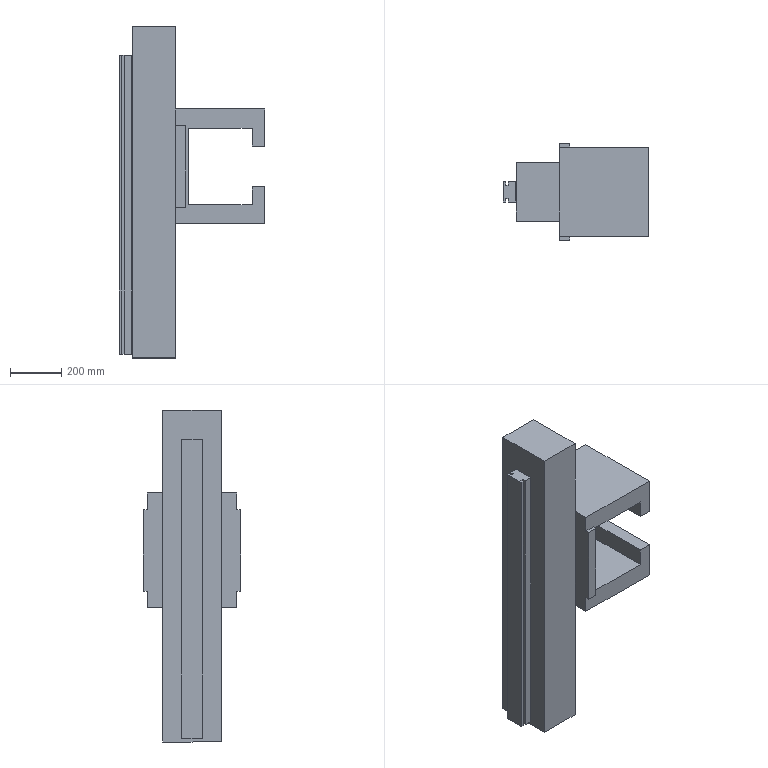Part | SolidWorks | features ICE 4, Extrusion 1 | 2 solids | 44 faces | box 571 x 380 x 1300 mm | volume 81618000 mm3 | plane 44
STEP:
#1=CARTESIAN_POINT('',(-175.,290.,550.));
#2=VERTEX_POINT('',#1);
#3=CARTESIAN_POINT('',(-345.,290.,550.));
#4=VERTEX_POINT('',#3);
#5=CARTESIAN_POINT('',(-345.,290.,550.));
#6=DIRECTION('',(-1.,0.,0.));
#7=VECTOR('',#6,1000.);
#8=LINE('',#5,#7);
#9=EDGE_CURVE('',#2,#4,#8,.T.);
#10=ORIENTED_EDGE('',*,*,#9,.F.);
#11=CARTESIAN_POINT('',(-175.,290.,225.));
#12=VERTEX_POINT('',#11);
#13=CARTESIAN_POINT('',(-175.,290.,-750.));
#14=DIRECTION('',(0.,0.,-1.));
#15=VECTOR('',#14,1000.);
#16=LINE('',#13,#15);
#17=EDGE_CURVE('',#2,#12,#16,.T.);
#18=ORIENTED_EDGE('',*,*,#17,.T.);
#19=CARTESIAN_POINT('',(-175.,290.,-225.));
#20=VERTEX_POINT('',#19);
#21=CARTESIAN_POINT('',(-175.,290.,-750.));
#22=DIRECTION('',(0.,0.,-1.));
#23=VECTOR('',#22,1000.);
#24=LINE('',#21,#23);
#25=EDGE_CURVE('',#12,#20,#24,.T.);
#26=ORIENTED_EDGE('',*,*,#25,.T.);
#27=CARTESIAN_POINT('',(-175.,290.,-750.));
#28=VERTEX_POINT('',#27);
#29=CARTESIAN_POINT('',(-175.,290.,-750.));
#30=DIRECTION('',(0.,0.,-1.));
#31=VECTOR('',#30,1000.);
#32=LINE('',#29,#31);
#33=EDGE_CURVE('',#20,#28,#32,.T.);
#34=ORIENTED_EDGE('',*,*,#33,.T.);
#35=CARTESIAN_POINT('',(-345.,290.,-750.));
#36=VERTEX_POINT('',#35);
#37=CARTESIAN_POINT('',(-345.,290.,-750.));
#38=DIRECTION('',(1.,0.,0.));
#39=VECTOR('',#38,1000.);
#40=LINE('',#37,#39);
#41=EDGE_CURVE('',#36,#28,#40,.T.);
#42=ORIENTED_EDGE('',*,*,#41,.F.);
#43=CARTESIAN_POINT('',(-345.,290.,-750.));
#44=DIRECTION('',(0.,0.,-1.));
#45=VECTOR('',#44,1000.);
#46=LINE('',#43,#45);
#47=EDGE_CURVE('',#4,#36,#46,.T.);
#48=ORIENTED_EDGE('',*,*,#47,.F.);
#49=EDGE_LOOP('',(#10,#18,#26,#34,#42,#48));
#50=FACE_OUTER_BOUND('',#49,.T.);
#51=CARTESIAN_POINT('',(-345.,290.,-750.));
#52=DIRECTION('',(0.,-1.,0.));
#53=DIRECTION('',(0.,0.,-1.));
#54=AXIS2_PLACEMENT_3D('',#51,#52,#53);
#55=PLANE('',#54);
#56=ADVANCED_FACE('',(#50),#55,.F.);
#57=CARTESIAN_POINT('',(-345.,60.,550.));
#58=VERTEX_POINT('',#57);
#59=CARTESIAN_POINT('',(-175.,60.,550.));
#60=VERTEX_POINT('',#59);
#61=CARTESIAN_POINT('',(-345.,60.,550.));
#62=DIRECTION('',(1.,0.,0.));
#63=VECTOR('',#62,1000.);
#64=LINE('',#61,#63);
#65=EDGE_CURVE('',#58,#60,#64,.T.);
#66=ORIENTED_EDGE('',*,*,#65,.F.);
#67=CARTESIAN_POINT('',(-345.,60.,-750.));
#68=VERTEX_POINT('',#67);
#69=CARTESIAN_POINT('',(-345.,60.,-750.));
#70=DIRECTION('',(0.,0.,1.));
#71=VECTOR('',#70,1000.);
#72=LINE('',#69,#71);
#73=EDGE_CURVE('',#68,#58,#72,.T.);
#74=ORIENTED_EDGE('',*,*,#73,.F.);
#75=CARTESIAN_POINT('',(-175.,60.,-750.));
#76=VERTEX_POINT('',#75);
#77=CARTESIAN_POINT('',(-345.,60.,-750.));
#78=DIRECTION('',(1.,0.,0.));
#79=VECTOR('',#78,1000.);
#80=LINE('',#77,#79);
#81=EDGE_CURVE('',#68,#76,#80,.T.);
#82=ORIENTED_EDGE('',*,*,#81,.T.);
#83=CARTESIAN_POINT('',(-175.,60.,-225.));
#84=VERTEX_POINT('',#83);
#85=CARTESIAN_POINT('',(-175.,60.,-750.));
#86=DIRECTION('',(0.,0.,1.));
#87=VECTOR('',#86,1000.);
#88=LINE('',#85,#87);
#89=EDGE_CURVE('',#76,#84,#88,.T.);
#90=ORIENTED_EDGE('',*,*,#89,.T.);
#91=CARTESIAN_POINT('',(-175.,60.,225.));
#92=VERTEX_POINT('',#91);
#93=CARTESIAN_POINT('',(-175.,60.,-750.));
#94=DIRECTION('',(0.,0.,1.));
#95=VECTOR('',#94,1000.);
#96=LINE('',#93,#95);
#97=EDGE_CURVE('',#84,#92,#96,.T.);
#98=ORIENTED_EDGE('',*,*,#97,.T.);
#99=CARTESIAN_POINT('',(-175.,60.,-750.));
#100=DIRECTION('',(0.,0.,1.));
#101=VECTOR('',#100,1000.);
#102=LINE('',#99,#101);
#103=EDGE_CURVE('',#92,#60,#102,.T.);
#104=ORIENTED_EDGE('',*,*,#103,.T.);
#105=EDGE_LOOP('',(#66,#74,#82,#90,#98,#104));
#106=FACE_OUTER_BOUND('',#105,.T.);
#107=CARTESIAN_POINT('',(-345.,60.,-750.));
#108=DIRECTION('',(0.,1.,0.));
#109=DIRECTION('',(0.,0.,1.));
#110=AXIS2_PLACEMENT_3D('',#107,#108,#109);
#111=PLANE('',#110);
#112=ADVANCED_FACE('',(#106),#111,.F.);
#113=ORIENTED_EDGE('',*,*,#73,.T.);
#114=CARTESIAN_POINT('',(-345.,0.,550.));
#115=DIRECTION('',(0.,1.,0.));
#116=VECTOR('',#115,1000.);
#117=LINE('',#114,#116);
#118=EDGE_CURVE('',#58,#4,#117,.T.);
#119=ORIENTED_EDGE('',*,*,#118,.T.);
#120=ORIENTED_EDGE('',*,*,#47,.T.);
#121=CARTESIAN_POINT('',(-345.,290.,-750.));
#122=DIRECTION('',(0.,-1.,0.));
#123=VECTOR('',#122,1000.);
#124=LINE('',#121,#123);
#125=EDGE_CURVE('',#36,#68,#124,.T.);
#126=ORIENTED_EDGE('',*,*,#125,.T.);
#127=EDGE_LOOP('',(#113,#119,#120,#126));
#128=FACE_OUTER_BOUND('',#127,.T.);
#129=CARTESIAN_POINT('',(-345.,0.,0.));
#130=DIRECTION('',(-1.,0.,0.));
#131=DIRECTION('',(0.,0.,1.));
#132=AXIS2_PLACEMENT_3D('',#129,#130,#131);
#133=PLANE('',#132);
#134=ADVANCED_FACE('',(#128),#133,.T.);
#135=CARTESIAN_POINT('',(-175.,0.,550.));
#136=DIRECTION('',(0.,1.,0.));
#137=VECTOR('',#136,1000.);
#138=LINE('',#135,#137);
#139=EDGE_CURVE('',#60,#2,#138,.T.);
#140=ORIENTED_EDGE('',*,*,#139,.F.);
#141=ORIENTED_EDGE('',*,*,#103,.F.);
#142=CARTESIAN_POINT('',(-175.,350.,225.));
#143=DIRECTION('',(0.,-1.,0.));
#144=VECTOR('',#143,1000.);
#145=LINE('',#142,#144);
#146=EDGE_CURVE('',#12,#92,#145,.T.);
#147=ORIENTED_EDGE('',*,*,#146,.F.);
#148=ORIENTED_EDGE('',*,*,#17,.F.);
#149=EDGE_LOOP('',(#140,#141,#147,#148));
#150=FACE_OUTER_BOUND('',#149,.T.);
#151=CARTESIAN_POINT('',(-175.,0.,0.));
#152=DIRECTION('',(-1.,0.,0.));
#153=DIRECTION('',(0.,0.,1.));
#154=AXIS2_PLACEMENT_3D('',#151,#152,#153);
#155=PLANE('',#154);
#156=ADVANCED_FACE('',(#150),#155,.F.);
#157=ORIENTED_EDGE('',*,*,#97,.F.);
#158=CARTESIAN_POINT('',(-175.,0.,-225.));
#159=VERTEX_POINT('',#158);
#160=CARTESIAN_POINT('',(-175.,350.,-225.));
#161=DIRECTION('',(0.,-1.,0.));
#162=VECTOR('',#161,1000.);
#163=LINE('',#160,#162);
#164=EDGE_CURVE('',#84,#159,#163,.T.);
#165=ORIENTED_EDGE('',*,*,#164,.T.);
#166=CARTESIAN_POINT('',(-175.,0.,-160.));
#167=VERTEX_POINT('',#166);
#168=CARTESIAN_POINT('',(-175.,0.,-225.));
#169=DIRECTION('',(0.,0.,1.));
#170=VECTOR('',#169,1000.);
#171=LINE('',#168,#170);
#172=EDGE_CURVE('',#159,#167,#171,.T.);
#173=ORIENTED_EDGE('',*,*,#172,.T.);
#174=CARTESIAN_POINT('',(-175.,-15.,-160.));
#175=VERTEX_POINT('',#174);
#176=CARTESIAN_POINT('',(-175.,365.,-160.));
#177=DIRECTION('',(0.,-1.,0.));
#178=VECTOR('',#177,1000.);
#179=LINE('',#176,#178);
#180=EDGE_CURVE('',#167,#175,#179,.T.);
#181=ORIENTED_EDGE('',*,*,#180,.T.);
#182=CARTESIAN_POINT('',(-175.,-15.,160.));
#183=VERTEX_POINT('',#182);
#184=CARTESIAN_POINT('',(-175.,-15.,-160.));
#185=DIRECTION('',(0.,0.,1.));
#186=VECTOR('',#185,1000.);
#187=LINE('',#184,#186);
#188=EDGE_CURVE('',#175,#183,#187,.T.);
#189=ORIENTED_EDGE('',*,*,#188,.T.);
#190=CARTESIAN_POINT('',(-175.,0.,160.));
#191=VERTEX_POINT('',#190);
#192=CARTESIAN_POINT('',(-175.,365.,160.));
#193=DIRECTION('',(0.,1.,0.));
#194=VECTOR('',#193,1000.);
#195=LINE('',#192,#194);
#196=EDGE_CURVE('',#183,#191,#195,.T.);
#197=ORIENTED_EDGE('',*,*,#196,.T.);
#198=CARTESIAN_POINT('',(-175.,0.,225.));
#199=VERTEX_POINT('',#198);
#200=CARTESIAN_POINT('',(-175.,0.,-225.));
#201=DIRECTION('',(0.,0.,1.));
#202=VECTOR('',#201,1000.);
#203=LINE('',#200,#202);
#204=EDGE_CURVE('',#191,#199,#203,.T.);
#205=ORIENTED_EDGE('',*,*,#204,.T.);
#206=CARTESIAN_POINT('',(-175.,350.,225.));
#207=DIRECTION('',(0.,-1.,0.));
#208=VECTOR('',#207,1000.);
#209=LINE('',#206,#208);
#210=EDGE_CURVE('',#92,#199,#209,.T.);
#211=ORIENTED_EDGE('',*,*,#210,.F.);
#212=EDGE_LOOP('',(#157,#165,#173,#181,#189,#197,#205,#211));
#213=FACE_OUTER_BOUND('',#212,.T.);
#214=CARTESIAN_POINT('',(-175.,350.,-225.));
#215=DIRECTION('',(1.,0.,0.));
#216=DIRECTION('',(0.,0.,-1.));
#217=AXIS2_PLACEMENT_3D('',#214,#215,#216);
#218=PLANE('',#217);
#219=ADVANCED_FACE('',(#213),#218,.F.);
#220=ORIENTED_EDGE('',*,*,#25,.F.);
#221=CARTESIAN_POINT('',(-175.,350.,225.));
#222=VERTEX_POINT('',#221);
#223=CARTESIAN_POINT('',(-175.,350.,225.));
#224=DIRECTION('',(0.,-1.,0.));
#225=VECTOR('',#224,1000.);
#226=LINE('',#223,#225);
#227=EDGE_CURVE('',#222,#12,#226,.T.);
#228=ORIENTED_EDGE('',*,*,#227,.F.);
#229=CARTESIAN_POINT('',(-175.,350.,160.));
#230=VERTEX_POINT('',#229);
#231=CARTESIAN_POINT('',(-175.,350.,-225.));
#232=DIRECTION('',(0.,0.,1.));
#233=VECTOR('',#232,1000.);
#234=LINE('',#231,#233);
#235=EDGE_CURVE('',#230,#222,#234,.T.);
#236=ORIENTED_EDGE('',*,*,#235,.F.);
#237=CARTESIAN_POINT('',(-175.,365.,160.));
#238=VERTEX_POINT('',#237);
#239=CARTESIAN_POINT('',(-175.,365.,160.));
#240=DIRECTION('',(0.,1.,0.));
#241=VECTOR('',#240,1000.);
#242=LINE('',#239,#241);
#243=EDGE_CURVE('',#230,#238,#242,.T.);
#244=ORIENTED_EDGE('',*,*,#243,.T.);
#245=CARTESIAN_POINT('',(-175.,365.,-160.));
#246=VERTEX_POINT('',#245);
#247=CARTESIAN_POINT('',(-175.,365.,-160.));
#248=DIRECTION('',(0.,0.,-1.));
#249=VECTOR('',#248,1000.);
#250=LINE('',#247,#249);
#251=EDGE_CURVE('',#238,#246,#250,.T.);
#252=ORIENTED_EDGE('',*,*,#251,.T.);
#253=CARTESIAN_POINT('',(-175.,350.,-160.));
#254=VERTEX_POINT('',#253);
#255=CARTESIAN_POINT('',(-175.,365.,-160.));
#256=DIRECTION('',(0.,-1.,0.));
#257=VECTOR('',#256,1000.);
#258=LINE('',#255,#257);
#259=EDGE_CURVE('',#246,#254,#258,.T.);
#260=ORIENTED_EDGE('',*,*,#259,.T.);
#261=CARTESIAN_POINT('',(-175.,350.,-225.));
#262=VERTEX_POINT('',#261);
#263=CARTESIAN_POINT('',(-175.,350.,-225.));
#264=DIRECTION('',(0.,0.,1.));
#265=VECTOR('',#264,1000.);
#266=LINE('',#263,#265);
#267=EDGE_CURVE('',#262,#254,#266,.T.);
#268=ORIENTED_EDGE('',*,*,#267,.F.);
#269=CARTESIAN_POINT('',(-175.,350.,-225.));
#270=DIRECTION('',(0.,-1.,0.));
#271=VECTOR('',#270,1000.);
#272=LINE('',#269,#271);
#273=EDGE_CURVE('',#262,#20,#272,.T.);
#274=ORIENTED_EDGE('',*,*,#273,.T.);
#275=EDGE_LOOP('',(#220,#228,#236,#244,#252,#260,#268,#274));
#276=FACE_OUTER_BOUND('',#275,.T.);
#277=CARTESIAN_POINT('',(-175.,350.,-225.));
#278=DIRECTION('',(1.,0.,0.));
#279=DIRECTION('',(0.,0.,-1.));
#280=AXIS2_PLACEMENT_3D('',#277,#278,#279);
#281=PLANE('',#280);
#282=ADVANCED_FACE('',(#276),#281,.F.);
#283=CARTESIAN_POINT('',(125.,0.,80.));
#284=VERTEX_POINT('',#283);
#285=CARTESIAN_POINT('',(125.,0.,150.));
#286=VERTEX_POINT('',#285);
#287=CARTESIAN_POINT('',(125.,0.,80.));
#288=DIRECTION('',(0.,0.,1.));
#289=VECTOR('',#288,1000.);
#290=LINE('',#287,#289);
#291=EDGE_CURVE('',#284,#286,#290,.T.);
#292=ORIENTED_EDGE('',*,*,#291,.T.);
#293=CARTESIAN_POINT('',(125.,350.,150.));
#294=VERTEX_POINT('',#293);
#295=CARTESIAN_POINT('',(125.,350.,150.));
#296=DIRECTION('',(0.,-1.,0.));
#297=VECTOR('',#296,1000.);
#298=LINE('',#295,#297);
#299=EDGE_CURVE('',#294,#286,#298,.T.);
#300=ORIENTED_EDGE('',*,*,#299,.F.);
#301=CARTESIAN_POINT('',(125.,350.,80.));
#302=VERTEX_POINT('',#301);
#303=CARTESIAN_POINT('',(125.,350.,80.));
#304=DIRECTION('',(0.,0.,1.));
#305=VECTOR('',#304,1000.);
#306=LINE('',#303,#305);
#307=EDGE_CURVE('',#302,#294,#306,.T.);
#308=ORIENTED_EDGE('',*,*,#307,.F.);
#309=CARTESIAN_POINT('',(125.,350.,80.));
#310=DIRECTION('',(0.,-1.,0.));
#311=VECTOR('',#310,1000.);
#312=LINE('',#309,#311);
#313=EDGE_CURVE('',#302,#284,#312,.T.);
#314=ORIENTED_EDGE('',*,*,#313,.T.);
#315=EDGE_LOOP('',(#292,#300,#308,#314));
#316=FACE_OUTER_BOUND('',#315,.T.);
#317=CARTESIAN_POINT('',(125.,350.,80.));
#318=DIRECTION('',(1.,0.,0.));
#319=DIRECTION('',(0.,0.,-1.));
#320=AXIS2_PLACEMENT_3D('',#317,#318,#319);
#321=PLANE('',#320);
#322=ADVANCED_FACE('',(#316),#321,.F.);
#323=CARTESIAN_POINT('',(-125.,0.,150.));
#324=VERTEX_POINT('',#323);
#325=CARTESIAN_POINT('',(-125.,0.,150.));
#326=DIRECTION('',(-1.,0.,0.));
#327=VECTOR('',#326,1000.);
#328=LINE('',#325,#327);
#329=EDGE_CURVE('',#286,#324,#328,.T.);
#330=ORIENTED_EDGE('',*,*,#329,.T.);
#331=CARTESIAN_POINT('',(-125.,350.,150.));
#332=VERTEX_POINT('',#331);
#333=CARTESIAN_POINT('',(-125.,350.,150.));
#334=DIRECTION('',(0.,-1.,0.));
#335=VECTOR('',#334,1000.);
#336=LINE('',#333,#335);
#337=EDGE_CURVE('',#332,#324,#336,.T.);
#338=ORIENTED_EDGE('',*,*,#337,.F.);
#339=CARTESIAN_POINT('',(-125.,350.,150.));
#340=DIRECTION('',(-1.,0.,0.));
#341=VECTOR('',#340,1000.);
#342=LINE('',#339,#341);
#343=EDGE_CURVE('',#294,#332,#342,.T.);
#344=ORIENTED_EDGE('',*,*,#343,.F.);
#345=ORIENTED_EDGE('',*,*,#299,.T.);
#346=EDGE_LOOP('',(#330,#338,#344,#345));
#347=FACE_OUTER_BOUND('',#346,.T.);
#348=CARTESIAN_POINT('',(-125.,350.,150.));
#349=DIRECTION('',(0.,0.,1.));
#350=DIRECTION('',(1.,0.,0.));
#351=AXIS2_PLACEMENT_3D('',#348,#349,#350);
#352=PLANE('',#351);
#353=ADVANCED_FACE('',(#347),#352,.F.);
#354=CARTESIAN_POINT('',(-125.,0.,-150.));
#355=VERTEX_POINT('',#354);
#356=CARTESIAN_POINT('',(-125.,0.,-150.));
#357=DIRECTION('',(0.,0.,-1.));
#358=VECTOR('',#357,1000.);
#359=LINE('',#356,#358);
#360=EDGE_CURVE('',#324,#355,#359,.T.);
#361=ORIENTED_EDGE('',*,*,#360,.T.);
#362=CARTESIAN_POINT('',(-125.,350.,-150.));
#363=VERTEX_POINT('',#362);
#364=CARTESIAN_POINT('',(-125.,350.,-150.));
#365=DIRECTION('',(0.,-1.,0.));
#366=VECTOR('',#365,1000.);
#367=LINE('',#364,#366);
#368=EDGE_CURVE('',#363,#355,#367,.T.);
#369=ORIENTED_EDGE('',*,*,#368,.F.);
#370=CARTESIAN_POINT('',(-125.,350.,-150.));
#371=DIRECTION('',(0.,0.,-1.));
#372=VECTOR('',#371,1000.);
#373=LINE('',#370,#372);
#374=EDGE_CURVE('',#332,#363,#373,.T.);
#375=ORIENTED_EDGE('',*,*,#374,.F.);
#376=ORIENTED_EDGE('',*,*,#337,.T.);
#377=EDGE_LOOP('',(#361,#369,#375,#376));
#378=FACE_OUTER_BOUND('',#377,.T.);
#379=CARTESIAN_POINT('',(-125.,350.,-150.));
#380=DIRECTION('',(-1.,0.,0.));
#381=DIRECTION('',(0.,0.,1.));
#382=AXIS2_PLACEMENT_3D('',#379,#380,#381);
#383=PLANE('',#382);
#384=ADVANCED_FACE('',(#378),#383,.F.);
#385=CARTESIAN_POINT('',(125.,0.,-150.));
#386=VERTEX_POINT('',#385);
#387=CARTESIAN_POINT('',(-125.,0.,-150.));
#388=DIRECTION('',(1.,0.,0.));
#389=VECTOR('',#388,1000.);
#390=LINE('',#387,#389);
#391=EDGE_CURVE('',#355,#386,#390,.T.);
#392=ORIENTED_EDGE('',*,*,#391,.T.);
#393=CARTESIAN_POINT('',(125.,350.,-150.));
#394=VERTEX_POINT('',#393);
#395=CARTESIAN_POINT('',(125.,350.,-150.));
#396=DIRECTION('',(0.,-1.,0.));
#397=VECTOR('',#396,1000.);
#398=LINE('',#395,#397);
#399=EDGE_CURVE('',#394,#386,#398,.T.);
#400=ORIENTED_EDGE('',*,*,#399,.F.);
#401=CARTESIAN_POINT('',(-125.,350.,-150.));
#402=DIRECTION('',(1.,0.,0.));
#403=VECTOR('',#402,1000.);
#404=LINE('',#401,#403);
#405=EDGE_CURVE('',#363,#394,#404,.T.);
#406=ORIENTED_EDGE('',*,*,#405,.F.);
#407=ORIENTED_EDGE('',*,*,#368,.T.);
#408=EDGE_LOOP('',(#392,#400,#406,#407));
#409=FACE_OUTER_BOUND('',#408,.T.);
#410=CARTESIAN_POINT('',(-125.,350.,-150.));
#411=DIRECTION('',(0.,0.,-1.));
#412=DIRECTION('',(-1.,0.,0.));
#413=AXIS2_PLACEMENT_3D('',#410,#411,#412);
#414=PLANE('',#413);
#415=ADVANCED_FACE('',(#409),#414,.F.);
#416=CARTESIAN_POINT('',(125.,0.,-80.));
#417=VERTEX_POINT('',#416);
#418=CARTESIAN_POINT('',(125.,0.,-150.));
#419=DIRECTION('',(0.,0.,1.));
#420=VECTOR('',#419,1000.);
#421=LINE('',#418,#420);
#422=EDGE_CURVE('',#386,#417,#421,.T.);
#423=ORIENTED_EDGE('',*,*,#422,.T.);
#424=CARTESIAN_POINT('',(125.,350.,-80.));
#425=VERTEX_POINT('',#424);
#426=CARTESIAN_POINT('',(125.,350.,-80.));
#427=DIRECTION('',(0.,-1.,0.));
#428=VECTOR('',#427,1000.);
#429=LINE('',#426,#428);
#430=EDGE_CURVE('',#425,#417,#429,.T.);
#431=ORIENTED_EDGE('',*,*,#430,.F.);
#432=CARTESIAN_POINT('',(125.,350.,-150.));
#433=DIRECTION('',(0.,0.,1.));
#434=VECTOR('',#433,1000.);
#435=LINE('',#432,#434);
#436=EDGE_CURVE('',#394,#425,#435,.T.);
#437=ORIENTED_EDGE('',*,*,#436,.F.);
#438=ORIENTED_EDGE('',*,*,#399,.T.);
#439=EDGE_LOOP('',(#423,#431,#437,#438));
#440=FACE_OUTER_BOUND('',#439,.T.);
#441=CARTESIAN_POINT('',(125.,350.,-150.));
#442=DIRECTION('',(1.,0.,0.));
#443=DIRECTION('',(0.,0.,-1.));
#444=AXIS2_PLACEMENT_3D('',#441,#442,#443);
#445=PLANE('',#444);
#446=ADVANCED_FACE('',(#440),#445,.F.);
#447=CARTESIAN_POINT('',(175.,0.,-80.));
#448=VERTEX_POINT('',#447);
#449=CARTESIAN_POINT('',(125.,0.,-80.));
#450=DIRECTION('',(1.,0.,0.));
#451=VECTOR('',#450,1000.);
#452=LINE('',#449,#451);
#453=EDGE_CURVE('',#417,#448,#452,.T.);
#454=ORIENTED_EDGE('',*,*,#453,.T.);
#455=CARTESIAN_POINT('',(175.,350.,-80.));
#456=VERTEX_POINT('',#455);
#457=CARTESIAN_POINT('',(175.,350.,-80.));
#458=DIRECTION('',(0.,-1.,0.));
#459=VECTOR('',#458,1000.);
#460=LINE('',#457,#459);
#461=EDGE_CURVE('',#456,#448,#460,.T.);
#462=ORIENTED_EDGE('',*,*,#461,.F.);
#463=CARTESIAN_POINT('',(125.,350.,-80.));
#464=DIRECTION('',(1.,0.,0.));
#465=VECTOR('',#464,1000.);
#466=LINE('',#463,#465);
#467=EDGE_CURVE('',#425,#456,#466,.T.);
#468=ORIENTED_EDGE('',*,*,#467,.F.);
#469=ORIENTED_EDGE('',*,*,#430,.T.);
#470=EDGE_LOOP('',(#454,#462,#468,#469));
#471=FACE_OUTER_BOUND('',#470,.T.);
#472=CARTESIAN_POINT('',(125.,350.,-80.));
#473=DIRECTION('',(0.,0.,-1.));
#474=DIRECTION('',(-1.,0.,0.));
#475=AXIS2_PLACEMENT_3D('',#472,#473,#474);
#476=PLANE('',#475);
#477=ADVANCED_FACE('',(#471),#476,.F.);
#478=CARTESIAN_POINT('',(175.,0.,-225.));
#479=VERTEX_POINT('',#478);
#480=CARTESIAN_POINT('',(175.,0.,-225.));
#481=DIRECTION('',(0.,0.,-1.));
#482=VECTOR('',#481,1000.);
#483=LINE('',#480,#482);
#484=EDGE_CURVE('',#448,#479,#483,.T.);
#485=ORIENTED_EDGE('',*,*,#484,.T.);
#486=CARTESIAN_POINT('',(175.,350.,-225.));
#487=VERTEX_POINT('',#486);
#488=CARTESIAN_POINT('',(175.,350.,-225.));
#489=DIRECTION('',(0.,-1.,0.));
#490=VECTOR('',#489,1000.);
#491=LINE('',#488,#490);
#492=EDGE_CURVE('',#487,#479,#491,.T.);
#493=ORIENTED_EDGE('',*,*,#492,.F.);
#494=CARTESIAN_POINT('',(175.,350.,-225.));
#495=DIRECTION('',(0.,0.,-1.));
#496=VECTOR('',#495,1000.);
#497=LINE('',#494,#496);
#498=EDGE_CURVE('',#456,#487,#497,.T.);
#499=ORIENTED_EDGE('',*,*,#498,.F.);
#500=ORIENTED_EDGE('',*,*,#461,.T.);
#501=EDGE_LOOP('',(#485,#493,#499,#500));
#502=FACE_OUTER_BOUND('',#501,.T.);
#503=CARTESIAN_POINT('',(175.,350.,-225.));
#504=DIRECTION('',(-1.,0.,0.));
#505=DIRECTION('',(0.,0.,1.));
#506=AXIS2_PLACEMENT_3D('',#503,#504,#505);
#507=PLANE('',#506);
#508=ADVANCED_FACE('',(#502),#507,.F.);
#509=CARTESIAN_POINT('',(-175.,0.,-225.));
#510=DIRECTION('',(-1.,0.,0.));
#511=VECTOR('',#510,1000.);
#512=LINE('',#509,#511);
#513=EDGE_CURVE('',#479,#159,#512,.T.);
#514=ORIENTED_EDGE('',*,*,#513,.T.);
#515=ORIENTED_EDGE('',*,*,#164,.F.);
#516=CARTESIAN_POINT('',(-175.,350.,-225.));
#517=DIRECTION('',(0.,-1.,0.));
#518=VECTOR('',#517,1000.);
#519=LINE('',#516,#518);
#520=EDGE_CURVE('',#20,#84,#519,.T.);
#521=ORIENTED_EDGE('',*,*,#520,.F.);
#522=ORIENTED_EDGE('',*,*,#273,.F.);
#523=CARTESIAN_POINT('',(-175.,350.,-225.));
#524=DIRECTION('',(-1.,0.,0.));
#525=VECTOR('',#524,1000.);
#526=LINE('',#523,#525);
#527=EDGE_CURVE('',#487,#262,#526,.T.);
#528=ORIENTED_EDGE('',*,*,#527,.F.);
#529=ORIENTED_EDGE('',*,*,#492,.T.);
#530=EDGE_LOOP('',(#514,#515,#521,#522,#528,#529));
#531=FACE_OUTER_BOUND('',#530,.T.);
#532=CARTESIAN_POINT('',(-175.,350.,-225.));
#533=DIRECTION('',(0.,0.,1.));
#534=DIRECTION('',(1.,0.,0.));
#535=AXIS2_PLACEMENT_3D('',#532,#533,#534);
#536=PLANE('',#535);
#537=ADVANCED_FACE('',(#531),#536,.F.);
#538=CARTESIAN_POINT('',(175.,0.,225.));
#539=VERTEX_POINT('',#538);
#540=CARTESIAN_POINT('',(-175.,0.,225.));
#541=DIRECTION('',(1.,0.,0.));
#542=VECTOR('',#541,1000.);
#543=LINE('',#540,#542);
#544=EDGE_CURVE('',#199,#539,#543,.T.);
#545=ORIENTED_EDGE('',*,*,#544,.T.);
#546=CARTESIAN_POINT('',(175.,350.,225.));
#547=VERTEX_POINT('',#546);
#548=CARTESIAN_POINT('',(175.,350.,225.));
#549=DIRECTION('',(0.,-1.,0.));
#550=VECTOR('',#549,1000.);
#551=LINE('',#548,#550);
#552=EDGE_CURVE('',#547,#539,#551,.T.);
#553=ORIENTED_EDGE('',*,*,#552,.F.);
#554=CARTESIAN_POINT('',(-175.,350.,225.));
#555=DIRECTION('',(1.,0.,0.));
#556=VECTOR('',#555,1000.);
#557=LINE('',#554,#556);
#558=EDGE_CURVE('',#222,#547,#557,.T.);
#559=ORIENTED_EDGE('',*,*,#558,.F.);
#560=ORIENTED_EDGE('',*,*,#227,.T.);
#561=ORIENTED_EDGE('',*,*,#146,.T.);
#562=ORIENTED_EDGE('',*,*,#210,.T.);
#563=EDGE_LOOP('',(#545,#553,#559,#560,#561,#562));
#564=FACE_OUTER_BOUND('',#563,.T.);
#565=CARTESIAN_POINT('',(-175.,350.,225.));
#566=DIRECTION('',(0.,0.,-1.));
#567=DIRECTION('',(-1.,0.,0.));
#568=AXIS2_PLACEMENT_3D('',#565,#566,#567);
#569=PLANE('',#568);
#570=ADVANCED_FACE('',(#564),#569,.F.);
#571=CARTESIAN_POINT('',(175.,0.,80.));
#572=VERTEX_POINT('',#571);
#573=CARTESIAN_POINT('',(175.,0.,80.));
#574=DIRECTION('',(0.,0.,-1.));
#575=VECTOR('',#574,1000.);
#576=LINE('',#573,#575);
#577=EDGE_CURVE('',#539,#572,#576,.T.);
#578=ORIENTED_EDGE('',*,*,#577,.T.);
#579=CARTESIAN_POINT('',(175.,350.,80.));
#580=VERTEX_POINT('',#579);
#581=CARTESIAN_POINT('',(175.,350.,80.));
#582=DIRECTION('',(0.,-1.,0.));
#583=VECTOR('',#582,1000.);
#584=LINE('',#581,#583);
#585=EDGE_CURVE('',#580,#572,#584,.T.);
#586=ORIENTED_EDGE('',*,*,#585,.F.);
#587=CARTESIAN_POINT('',(175.,350.,80.));
#588=DIRECTION('',(0.,0.,-1.));
#589=VECTOR('',#588,1000.);
#590=LINE('',#587,#589);
#591=EDGE_CURVE('',#547,#580,#590,.T.);
#592=ORIENTED_EDGE('',*,*,#591,.F.);
#593=ORIENTED_EDGE('',*,*,#552,.T.);
#594=EDGE_LOOP('',(#578,#586,#592,#593));
#595=FACE_OUTER_BOUND('',#594,.T.);
#596=CARTESIAN_POINT('',(175.,350.,80.));
#597=DIRECTION('',(-1.,0.,0.));
#598=DIRECTION('',(0.,0.,1.));
#599=AXIS2_PLACEMENT_3D('',#596,#597,#598);
#600=PLANE('',#599);
#601=ADVANCED_FACE('',(#595),#600,.F.);
#602=CARTESIAN_POINT('',(125.,0.,80.));
#603=DIRECTION('',(-1.,0.,0.));
#604=VECTOR('',#603,1000.);
#605=LINE('',#602,#604);
#606=EDGE_CURVE('',#572,#284,#605,.T.);
#607=ORIENTED_EDGE('',*,*,#606,.T.);
#608=ORIENTED_EDGE('',*,*,#313,.F.);
#609=CARTESIAN_POINT('',(125.,350.,80.));
#610=DIRECTION('',(-1.,0.,0.));
#611=VECTOR('',#610,1000.);
#612=LINE('',#609,#611);
#613=EDGE_CURVE('',#580,#302,#612,.T.);
#614=ORIENTED_EDGE('',*,*,#613,.F.);
#615=ORIENTED_EDGE('',*,*,#585,.T.);
#616=EDGE_LOOP('',(#607,#608,#614,#615));
#617=FACE_OUTER_BOUND('',#616,.T.);
#618=CARTESIAN_POINT('',(125.,350.,80.));
#619=DIRECTION('',(0.,0.,1.));
#620=DIRECTION('',(1.,0.,0.));
#621=AXIS2_PLACEMENT_3D('',#618,#619,#620);
#622=PLANE('',#621);
#623=ADVANCED_FACE('',(#617),#622,.F.);
#624=CARTESIAN_POINT('',(-135.,350.,160.));
#625=VERTEX_POINT('',#624);
#626=CARTESIAN_POINT('',(0.,350.,160.));
#627=DIRECTION('',(1.,0.,0.));
#628=VECTOR('',#627,1000.);
#629=LINE('',#626,#628);
#630=EDGE_CURVE('',#230,#625,#629,.T.);
#631=ORIENTED_EDGE('',*,*,#630,.F.);
#632=ORIENTED_EDGE('',*,*,#235,.T.);
#633=ORIENTED_EDGE('',*,*,#558,.T.);
#634=ORIENTED_EDGE('',*,*,#591,.T.);
#635=ORIENTED_EDGE('',*,*,#613,.T.);
#636=ORIENTED_EDGE('',*,*,#307,.T.);
#637=ORIENTED_EDGE('',*,*,#343,.T.);
#638=ORIENTED_EDGE('',*,*,#374,.T.);
#639=ORIENTED_EDGE('',*,*,#405,.T.);
#640=ORIENTED_EDGE('',*,*,#436,.T.);
#641=ORIENTED_EDGE('',*,*,#467,.T.);
#642=ORIENTED_EDGE('',*,*,#498,.T.);
#643=ORIENTED_EDGE('',*,*,#527,.T.);
#644=ORIENTED_EDGE('',*,*,#267,.T.);
#645=CARTESIAN_POINT('',(-135.,350.,-160.));
#646=VERTEX_POINT('',#645);
#647=CARTESIAN_POINT('',(0.,350.,-160.));
#648=DIRECTION('',(-1.,0.,0.));
#649=VECTOR('',#648,1000.);
#650=LINE('',#647,#649);
#651=EDGE_CURVE('',#646,#254,#650,.T.);
#652=ORIENTED_EDGE('',*,*,#651,.F.);
#653=CARTESIAN_POINT('',(-135.,350.,0.));
#654=DIRECTION('',(0.,0.,1.));
#655=VECTOR('',#654,1000.);
#656=LINE('',#653,#655);
#657=EDGE_CURVE('',#646,#625,#656,.T.);
#658=ORIENTED_EDGE('',*,*,#657,.T.);
#659=EDGE_LOOP('',(#631,#632,#633,#634,#635,#636,#637,#638,#639,#640,#641,#642,#643,#644,#652,#658));
#660=FACE_OUTER_BOUND('',#659,.T.);
#661=CARTESIAN_POINT('',(0.,350.,0.));
#662=DIRECTION('',(0.,1.,0.));
#663=DIRECTION('',(0.,0.,1.));
#664=AXIS2_PLACEMENT_3D('',#661,#662,#663);
#665=PLANE('',#664);
#666=ADVANCED_FACE('',(#660),#665,.T.);
#667=ORIENTED_EDGE('',*,*,#204,.F.);
#668=CARTESIAN_POINT('',(-135.,0.,160.));
#669=VERTEX_POINT('',#668);
#670=CARTESIAN_POINT('',(0.,0.,160.));
#671=DIRECTION('',(1.,0.,0.));
#672=VECTOR('',#671,1000.);
#673=LINE('',#670,#672);
#674=EDGE_CURVE('',#191,#669,#673,.T.);
#675=ORIENTED_EDGE('',*,*,#674,.T.);
#676=CARTESIAN_POINT('',(-135.,0.,-160.));
#677=VERTEX_POINT('',#676);
#678=CARTESIAN_POINT('',(-135.,0.,0.));
#679=DIRECTION('',(0.,0.,1.));
#680=VECTOR('',#679,1000.);
#681=LINE('',#678,#680);
#682=EDGE_CURVE('',#677,#669,#681,.T.);
#683=ORIENTED_EDGE('',*,*,#682,.F.);
#684=CARTESIAN_POINT('',(0.,0.,-160.));
#685=DIRECTION('',(-1.,0.,0.));
#686=VECTOR('',#685,1000.);
#687=LINE('',#684,#686);
#688=EDGE_CURVE('',#677,#167,#687,.T.);
#689=ORIENTED_EDGE('',*,*,#688,.T.);
#690=ORIENTED_EDGE('',*,*,#172,.F.);
#691=ORIENTED_EDGE('',*,*,#513,.F.);
#692=ORIENTED_EDGE('',*,*,#484,.F.);
#693=ORIENTED_EDGE('',*,*,#453,.F.);
#694=ORIENTED_EDGE('',*,*,#422,.F.);
#695=ORIENTED_EDGE('',*,*,#391,.F.);
#696=ORIENTED_EDGE('',*,*,#360,.F.);
#697=ORIENTED_EDGE('',*,*,#329,.F.);
#698=ORIENTED_EDGE('',*,*,#291,.F.);
#699=ORIENTED_EDGE('',*,*,#606,.F.);
#700=ORIENTED_EDGE('',*,*,#577,.F.);
#701=ORIENTED_EDGE('',*,*,#544,.F.);
#702=EDGE_LOOP('',(#667,#675,#683,#689,#690,#691,#692,#693,#694,#695,#696,#697,#698,#699,#700,#701));
#703=FACE_OUTER_BOUND('',#702,.T.);
#704=CARTESIAN_POINT('',(0.,0.,0.));
#705=DIRECTION('',(0.,1.,0.));
#706=DIRECTION('',(0.,0.,1.));
#707=AXIS2_PLACEMENT_3D('',#704,#705,#706);
#708=PLANE('',#707);
#709=ADVANCED_FACE('',(#703),#708,.F.);
#710=ORIENTED_EDGE('',*,*,#188,.F.);
#711=CARTESIAN_POINT('',(-135.,-15.,-160.));
#712=VERTEX_POINT('',#711);
#713=CARTESIAN_POINT('',(-135.,-15.,-160.));
#714=DIRECTION('',(-1.,0.,0.));
#715=VECTOR('',#714,1000.);
#716=LINE('',#713,#715);
#717=EDGE_CURVE('',#712,#175,#716,.T.);
#718=ORIENTED_EDGE('',*,*,#717,.F.);
#719=CARTESIAN_POINT('',(-135.,-15.,160.));
#720=VERTEX_POINT('',#719);
#721=CARTESIAN_POINT('',(-135.,-15.,-160.));
#722=DIRECTION('',(0.,0.,1.));
#723=VECTOR('',#722,1000.);
#724=LINE('',#721,#723);
#725=EDGE_CURVE('',#712,#720,#724,.T.);
#726=ORIENTED_EDGE('',*,*,#725,.T.);
#727=CARTESIAN_POINT('',(-135.,-15.,160.));
#728=DIRECTION('',(-1.,0.,0.));
#729=VECTOR('',#728,1000.);
#730=LINE('',#727,#729);
#731=EDGE_CURVE('',#720,#183,#730,.T.);
#732=ORIENTED_EDGE('',*,*,#731,.T.);
#733=EDGE_LOOP('',(#710,#718,#726,#732));
#734=FACE_OUTER_BOUND('',#733,.T.);
#735=CARTESIAN_POINT('',(-135.,-15.,-160.));
#736=DIRECTION('',(0.,-1.,0.));
#737=DIRECTION('',(0.,0.,-1.));
#738=AXIS2_PLACEMENT_3D('',#735,#736,#737);
#739=PLANE('',#738);
#740=ADVANCED_FACE('',(#734),#739,.T.);
#741=CARTESIAN_POINT('',(-135.,365.,-160.));
#742=DIRECTION('',(0.,-1.,0.));
#743=VECTOR('',#742,1000.);
#744=LINE('',#741,#743);
#745=EDGE_CURVE('',#677,#712,#744,.T.);
#746=ORIENTED_EDGE('',*,*,#745,.F.);
#747=ORIENTED_EDGE('',*,*,#682,.T.);
#748=CARTESIAN_POINT('',(-135.,365.,160.));
#749=DIRECTION('',(0.,1.,0.));
#750=VECTOR('',#749,1000.);
#751=LINE('',#748,#750);
#752=EDGE_CURVE('',#720,#669,#751,.T.);
#753=ORIENTED_EDGE('',*,*,#752,.F.);
#754=ORIENTED_EDGE('',*,*,#725,.F.);
#755=EDGE_LOOP('',(#746,#747,#753,#754));
#756=FACE_OUTER_BOUND('',#755,.T.);
#757=CARTESIAN_POINT('',(-135.,0.,0.));
#758=DIRECTION('',(-1.,0.,0.));
#759=DIRECTION('',(0.,0.,1.));
#760=AXIS2_PLACEMENT_3D('',#757,#758,#759);
#761=PLANE('',#760);
#762=ADVANCED_FACE('',(#756),#761,.F.);
#763=ORIENTED_EDGE('',*,*,#688,.F.);
#764=ORIENTED_EDGE('',*,*,#745,.T.);
#765=ORIENTED_EDGE('',*,*,#717,.T.);
#766=ORIENTED_EDGE('',*,*,#180,.F.);
#767=EDGE_LOOP('',(#763,#764,#765,#766));
#768=FACE_OUTER_BOUND('',#767,.T.);
#769=CARTESIAN_POINT('',(-135.,365.,-160.));
#770=DIRECTION('',(0.,0.,-1.));
#771=DIRECTION('',(0.,1.,0.));
#772=AXIS2_PLACEMENT_3D('',#769,#770,#771);
#773=PLANE('',#772);
#774=ADVANCED_FACE('',(#768),#773,.T.);
#775=ORIENTED_EDGE('',*,*,#674,.F.);
#776=ORIENTED_EDGE('',*,*,#196,.F.);
#777=ORIENTED_EDGE('',*,*,#731,.F.);
#778=ORIENTED_EDGE('',*,*,#752,.T.);
#779=EDGE_LOOP('',(#775,#776,#777,#778));
#780=FACE_OUTER_BOUND('',#779,.T.);
#781=CARTESIAN_POINT('',(-135.,365.,160.));
#782=DIRECTION('',(0.,0.,1.));
#783=DIRECTION('',(0.,-1.,0.));
#784=AXIS2_PLACEMENT_3D('',#781,#782,#783);
#785=PLANE('',#784);
#786=ADVANCED_FACE('',(#780),#785,.T.);
#787=ORIENTED_EDGE('',*,*,#243,.F.);
#788=ORIENTED_EDGE('',*,*,#630,.T.);
#789=CARTESIAN_POINT('',(-135.,365.,160.));
#790=VERTEX_POINT('',#789);
#791=CARTESIAN_POINT('',(-135.,365.,160.));
#792=DIRECTION('',(0.,1.,0.));
#793=VECTOR('',#792,1000.);
#794=LINE('',#791,#793);
#795=EDGE_CURVE('',#625,#790,#794,.T.);
#796=ORIENTED_EDGE('',*,*,#795,.T.);
#797=CARTESIAN_POINT('',(-135.,365.,160.));
#798=DIRECTION('',(-1.,0.,0.));
#799=VECTOR('',#798,1000.);
#800=LINE('',#797,#799);
#801=EDGE_CURVE('',#790,#238,#800,.T.);
#802=ORIENTED_EDGE('',*,*,#801,.T.);
#803=EDGE_LOOP('',(#787,#788,#796,#802));
#804=FACE_OUTER_BOUND('',#803,.T.);
#805=CARTESIAN_POINT('',(-135.,365.,160.));
#806=DIRECTION('',(0.,0.,1.));
#807=DIRECTION('',(0.,-1.,0.));
#808=AXIS2_PLACEMENT_3D('',#805,#806,#807);
#809=PLANE('',#808);
#810=ADVANCED_FACE('',(#804),#809,.T.);
#811=CARTESIAN_POINT('',(-135.,365.,-160.));
#812=VERTEX_POINT('',#811);
#813=CARTESIAN_POINT('',(-135.,365.,-160.));
#814=DIRECTION('',(0.,-1.,0.));
#815=VECTOR('',#814,1000.);
#816=LINE('',#813,#815);
#817=EDGE_CURVE('',#812,#646,#816,.T.);
#818=ORIENTED_EDGE('',*,*,#817,.T.);
#819=ORIENTED_EDGE('',*,*,#651,.T.);
#820=ORIENTED_EDGE('',*,*,#259,.F.);
#821=CARTESIAN_POINT('',(-135.,365.,-160.));
#822=DIRECTION('',(-1.,0.,0.));
#823=VECTOR('',#822,1000.);
#824=LINE('',#821,#823);
#825=EDGE_CURVE('',#812,#246,#824,.T.);
#826=ORIENTED_EDGE('',*,*,#825,.F.);
#827=EDGE_LOOP('',(#818,#819,#820,#826));
#828=FACE_OUTER_BOUND('',#827,.T.);
#829=CARTESIAN_POINT('',(-135.,365.,-160.));
#830=DIRECTION('',(0.,0.,-1.));
#831=DIRECTION('',(0.,1.,0.));
#832=AXIS2_PLACEMENT_3D('',#829,#830,#831);
#833=PLANE('',#832);
#834=ADVANCED_FACE('',(#828),#833,.T.);
#835=ORIENTED_EDGE('',*,*,#251,.F.);
#836=ORIENTED_EDGE('',*,*,#801,.F.);
#837=CARTESIAN_POINT('',(-135.,365.,-160.));
#838=DIRECTION('',(0.,0.,-1.));
#839=VECTOR('',#838,1000.);
#840=LINE('',#837,#839);
#841=EDGE_CURVE('',#790,#812,#840,.T.);
#842=ORIENTED_EDGE('',*,*,#841,.T.);
#843=ORIENTED_EDGE('',*,*,#825,.T.);
#844=EDGE_LOOP('',(#835,#836,#842,#843));
#845=FACE_OUTER_BOUND('',#844,.T.);
#846=CARTESIAN_POINT('',(-135.,365.,-160.));
#847=DIRECTION('',(0.,1.,0.));
#848=DIRECTION('',(0.,0.,1.));
#849=AXIS2_PLACEMENT_3D('',#846,#847,#848);
#850=PLANE('',#849);
#851=ADVANCED_FACE('',(#845),#850,.T.);
#852=ORIENTED_EDGE('',*,*,#657,.F.);
#853=ORIENTED_EDGE('',*,*,#817,.F.);
#854=ORIENTED_EDGE('',*,*,#841,.F.);
#855=ORIENTED_EDGE('',*,*,#795,.F.);
#856=EDGE_LOOP('',(#852,#853,#854,#855));
#857=FACE_OUTER_BOUND('',#856,.T.);
#858=CARTESIAN_POINT('',(-135.,0.,0.));
#859=DIRECTION('',(-1.,0.,0.));
#860=DIRECTION('',(0.,0.,1.));
#861=AXIS2_PLACEMENT_3D('',#858,#859,#860);
#862=PLANE('',#861);
#863=ADVANCED_FACE('',(#857),#862,.F.);
#864=ORIENTED_EDGE('',*,*,#33,.F.);
#865=ORIENTED_EDGE('',*,*,#520,.T.);
#866=ORIENTED_EDGE('',*,*,#89,.F.);
#867=CARTESIAN_POINT('',(-175.,290.,-750.));
#868=DIRECTION('',(0.,-1.,0.));
#869=VECTOR('',#868,1000.);
#870=LINE('',#867,#869);
#871=EDGE_CURVE('',#28,#76,#870,.T.);
#872=ORIENTED_EDGE('',*,*,#871,.F.);
#873=EDGE_LOOP('',(#864,#865,#866,#872));
#874=FACE_OUTER_BOUND('',#873,.T.);
#875=CARTESIAN_POINT('',(-175.,0.,0.));
#876=DIRECTION('',(-1.,0.,0.));
#877=DIRECTION('',(0.,0.,1.));
#878=AXIS2_PLACEMENT_3D('',#875,#876,#877);
#879=PLANE('',#878);
#880=ADVANCED_FACE('',(#874),#879,.F.);
#881=ORIENTED_EDGE('',*,*,#871,.T.);
#882=ORIENTED_EDGE('',*,*,#81,.F.);
#883=ORIENTED_EDGE('',*,*,#125,.F.);
#884=ORIENTED_EDGE('',*,*,#41,.T.);
#885=EDGE_LOOP('',(#881,#882,#883,#884));
#886=FACE_OUTER_BOUND('',#885,.T.);
#887=CARTESIAN_POINT('',(-345.,290.,-750.));
#888=DIRECTION('',(0.,0.,1.));
#889=DIRECTION('',(0.,-1.,0.));
#890=AXIS2_PLACEMENT_3D('',#887,#888,#889);
#891=PLANE('',#890);
#892=ADVANCED_FACE('',(#886),#891,.F.);
#893=ORIENTED_EDGE('',*,*,#65,.T.);
#894=ORIENTED_EDGE('',*,*,#139,.T.);
#895=ORIENTED_EDGE('',*,*,#9,.T.);
#896=ORIENTED_EDGE('',*,*,#118,.F.);
#897=EDGE_LOOP('',(#893,#894,#895,#896));
#898=FACE_OUTER_BOUND('',#897,.T.);
#899=CARTESIAN_POINT('',(0.,0.,550.));
#900=DIRECTION('',(0.,0.,1.));
#901=DIRECTION('',(1.,0.,0.));
#902=AXIS2_PLACEMENT_3D('',#899,#900,#901);
#903=PLANE('',#902);
#904=ADVANCED_FACE('',(#898),#903,.T.);
#905=CLOSED_SHELL('',(#56,#112,#134,#156,#219,#282,#322,#353,#384,#415,#446,#477,#508,#537,#570,#601,#623,#666,#709,#740,#762,#774,#786,#810,#834,#851,#863,#880,#892,#904));
#906=MANIFOLD_SOLID_BREP('',#905);
#907=CARTESIAN_POINT('',(-386.,135.,-735.));
#908=VERTEX_POINT('',#907);
#909=CARTESIAN_POINT('',(-396.,135.,-735.));
#910=VERTEX_POINT('',#909);
#911=CARTESIAN_POINT('',(-386.,135.,-735.));
#912=DIRECTION('',(-1.,0.,0.));
#913=VECTOR('',#912,1000.);
#914=LINE('',#911,#913);
#915=EDGE_CURVE('',#908,#910,#914,.T.);
#916=ORIENTED_EDGE('',*,*,#915,.F.);
#917=CARTESIAN_POINT('',(-386.,135.,435.));
#918=VERTEX_POINT('',#917);
#919=CARTESIAN_POINT('',(-386.,135.,435.));
#920=DIRECTION('',(0.,0.,-1.));
#921=VECTOR('',#920,1000.);
#922=LINE('',#919,#921);
#923=EDGE_CURVE('',#918,#908,#922,.T.);
#924=ORIENTED_EDGE('',*,*,#923,.F.);
#925=CARTESIAN_POINT('',(-396.,135.,435.));
#926=VERTEX_POINT('',#925);
#927=CARTESIAN_POINT('',(-386.,135.,435.));
#928=DIRECTION('',(-1.,0.,0.));
#929=VECTOR('',#928,1000.);
#930=LINE('',#927,#929);
#931=EDGE_CURVE('',#918,#926,#930,.T.);
#932=ORIENTED_EDGE('',*,*,#931,.T.);
#933=CARTESIAN_POINT('',(-396.,135.,435.));
#934=DIRECTION('',(0.,0.,-1.));
#935=VECTOR('',#934,1000.);
#936=LINE('',#933,#935);
#937=EDGE_CURVE('',#926,#910,#936,.T.);
#938=ORIENTED_EDGE('',*,*,#937,.T.);
#939=EDGE_LOOP('',(#916,#924,#932,#938));
#940=FACE_OUTER_BOUND('',#939,.T.);
#941=CARTESIAN_POINT('',(-386.,135.,435.));
#942=DIRECTION('',(0.,-1.,0.));
#943=DIRECTION('',(0.,0.,-1.));
#944=AXIS2_PLACEMENT_3D('',#941,#942,#943);
#945=PLANE('',#944);
#946=ADVANCED_FACE('',(#940),#945,.T.);
#947=CARTESIAN_POINT('',(-386.,150.,-735.));
#948=VERTEX_POINT('',#947);
#949=CARTESIAN_POINT('',(-386.,135.,-735.));
#950=DIRECTION('',(0.,-1.,0.));
#951=VECTOR('',#950,1000.);
#952=LINE('',#949,#951);
#953=EDGE_CURVE('',#948,#908,#952,.T.);
#954=ORIENTED_EDGE('',*,*,#953,.F.);
#955=CARTESIAN_POINT('',(-386.,150.,435.));
#956=VERTEX_POINT('',#955);
#957=CARTESIAN_POINT('',(-386.,150.,435.));
#958=DIRECTION('',(0.,0.,-1.));
#959=VECTOR('',#958,1000.);
#960=LINE('',#957,#959);
#961=EDGE_CURVE('',#956,#948,#960,.T.);
#962=ORIENTED_EDGE('',*,*,#961,.F.);
#963=CARTESIAN_POINT('',(-386.,135.,435.));
#964=DIRECTION('',(0.,-1.,0.));
#965=VECTOR('',#964,1000.);
#966=LINE('',#963,#965);
#967=EDGE_CURVE('',#956,#918,#966,.T.);
#968=ORIENTED_EDGE('',*,*,#967,.T.);
#969=ORIENTED_EDGE('',*,*,#923,.T.);
#970=EDGE_LOOP('',(#954,#962,#968,#969));
#971=FACE_OUTER_BOUND('',#970,.T.);
#972=CARTESIAN_POINT('',(-386.,135.,435.));
#973=DIRECTION('',(1.,0.,0.));
#974=DIRECTION('',(0.,0.,-1.));
#975=AXIS2_PLACEMENT_3D('',#972,#973,#974);
#976=PLANE('',#975);
#977=ADVANCED_FACE('',(#971),#976,.T.);
#978=CARTESIAN_POINT('',(-376.,150.,-735.));
#979=VERTEX_POINT('',#978);
#980=CARTESIAN_POINT('',(-386.,150.,-735.));
#981=DIRECTION('',(-1.,0.,0.));
#982=VECTOR('',#981,1000.);
#983=LINE('',#980,#982);
#984=EDGE_CURVE('',#979,#948,#983,.T.);
#985=ORIENTED_EDGE('',*,*,#984,.F.);
#986=CARTESIAN_POINT('',(-376.,150.,435.));
#987=VERTEX_POINT('',#986);
#988=CARTESIAN_POINT('',(-376.,150.,435.));
#989=DIRECTION('',(0.,0.,-1.));
#990=VECTOR('',#989,1000.);
#991=LINE('',#988,#990);
#992=EDGE_CURVE('',#987,#979,#991,.T.);
#993=ORIENTED_EDGE('',*,*,#992,.F.);
#994=CARTESIAN_POINT('',(-386.,150.,435.));
#995=DIRECTION('',(-1.,0.,0.));
#996=VECTOR('',#995,1000.);
#997=LINE('',#994,#996);
#998=EDGE_CURVE('',#987,#956,#997,.T.);
#999=ORIENTED_EDGE('',*,*,#998,.T.);
#1000=ORIENTED_EDGE('',*,*,#961,.T.);
#1001=EDGE_LOOP('',(#985,#993,#999,#1000));
#1002=FACE_OUTER_BOUND('',#1001,.T.);
#1003=CARTESIAN_POINT('',(-386.,150.,435.));
#1004=DIRECTION('',(0.,-1.,0.));
#1005=DIRECTION('',(0.,0.,-1.));
#1006=AXIS2_PLACEMENT_3D('',#1003,#1004,#1005);
#1007=PLANE('',#1006);
#1008=ADVANCED_FACE('',(#1002),#1007,.T.);
#1009=CARTESIAN_POINT('',(-376.,135.,-735.));
#1010=VERTEX_POINT('',#1009);
#1011=CARTESIAN_POINT('',(-376.,150.,-735.));
#1012=DIRECTION('',(0.,1.,0.));
#1013=VECTOR('',#1012,1000.);
#1014=LINE('',#1011,#1013);
#1015=EDGE_CURVE('',#1010,#979,#1014,.T.);
#1016=ORIENTED_EDGE('',*,*,#1015,.F.);
#1017=CARTESIAN_POINT('',(-376.,135.,435.));
#1018=VERTEX_POINT('',#1017);
#1019=CARTESIAN_POINT('',(-376.,135.,435.));
#1020=DIRECTION('',(0.,0.,-1.));
#1021=VECTOR('',#1020,1000.);
#1022=LINE('',#1019,#1021);
#1023=EDGE_CURVE('',#1018,#1010,#1022,.T.);
#1024=ORIENTED_EDGE('',*,*,#1023,.F.);
#1025=CARTESIAN_POINT('',(-376.,150.,435.));
#1026=DIRECTION('',(0.,1.,0.));
#1027=VECTOR('',#1026,1000.);
#1028=LINE('',#1025,#1027);
#1029=EDGE_CURVE('',#1018,#987,#1028,.T.);
#1030=ORIENTED_EDGE('',*,*,#1029,.T.);
#1031=ORIENTED_EDGE('',*,*,#992,.T.);
#1032=EDGE_LOOP('',(#1016,#1024,#1030,#1031));
#1033=FACE_OUTER_BOUND('',#1032,.T.);
#1034=CARTESIAN_POINT('',(-376.,150.,435.));
#1035=DIRECTION('',(-1.,0.,0.));
#1036=DIRECTION('',(0.,0.,1.));
#1037=AXIS2_PLACEMENT_3D('',#1034,#1035,#1036);
#1038=PLANE('',#1037);
#1039=ADVANCED_FACE('',(#1033),#1038,.T.);
#1040=CARTESIAN_POINT('',(-346.,135.,-735.));
#1041=VERTEX_POINT('',#1040);
#1042=CARTESIAN_POINT('',(-346.,135.,-735.));
#1043=DIRECTION('',(-1.,0.,0.));
#1044=VECTOR('',#1043,1000.);
#1045=LINE('',#1042,#1044);
#1046=EDGE_CURVE('',#1041,#1010,#1045,.T.);
#1047=ORIENTED_EDGE('',*,*,#1046,.F.);
#1048=CARTESIAN_POINT('',(-346.,135.,435.));
#1049=VERTEX_POINT('',#1048);
#1050=CARTESIAN_POINT('',(-346.,135.,435.));
#1051=DIRECTION('',(0.,0.,-1.));
#1052=VECTOR('',#1051,1000.);
#1053=LINE('',#1050,#1052);
#1054=EDGE_CURVE('',#1049,#1041,#1053,.T.);
#1055=ORIENTED_EDGE('',*,*,#1054,.F.);
#1056=CARTESIAN_POINT('',(-346.,135.,435.));
#1057=DIRECTION('',(-1.,0.,0.));
#1058=VECTOR('',#1057,1000.);
#1059=LINE('',#1056,#1058);
#1060=EDGE_CURVE('',#1049,#1018,#1059,.T.);
#1061=ORIENTED_EDGE('',*,*,#1060,.T.);
#1062=ORIENTED_EDGE('',*,*,#1023,.T.);
#1063=EDGE_LOOP('',(#1047,#1055,#1061,#1062));
#1064=FACE_OUTER_BOUND('',#1063,.T.);
#1065=CARTESIAN_POINT('',(-346.,135.,435.));
#1066=DIRECTION('',(0.,-1.,0.));
#1067=DIRECTION('',(0.,0.,-1.));
#1068=AXIS2_PLACEMENT_3D('',#1065,#1066,#1067);
#1069=PLANE('',#1068);
#1070=ADVANCED_FACE('',(#1064),#1069,.T.);
#1071=CARTESIAN_POINT('',(-346.,215.,-735.));
#1072=VERTEX_POINT('',#1071);
#1073=CARTESIAN_POINT('',(-346.,215.,-735.));
#1074=DIRECTION('',(0.,-1.,0.));
#1075=VECTOR('',#1074,1000.);
#1076=LINE('',#1073,#1075);
#1077=EDGE_CURVE('',#1072,#1041,#1076,.T.);
#1078=ORIENTED_EDGE('',*,*,#1077,.F.);
#1079=CARTESIAN_POINT('',(-346.,215.,435.));
#1080=VERTEX_POINT('',#1079);
#1081=CARTESIAN_POINT('',(-346.,215.,435.));
#1082=DIRECTION('',(0.,0.,-1.));
#1083=VECTOR('',#1082,1000.);
#1084=LINE('',#1081,#1083);
#1085=EDGE_CURVE('',#1080,#1072,#1084,.T.);
#1086=ORIENTED_EDGE('',*,*,#1085,.F.);
#1087=CARTESIAN_POINT('',(-346.,215.,435.));
#1088=DIRECTION('',(0.,-1.,0.));
#1089=VECTOR('',#1088,1000.);
#1090=LINE('',#1087,#1089);
#1091=EDGE_CURVE('',#1080,#1049,#1090,.T.);
#1092=ORIENTED_EDGE('',*,*,#1091,.T.);
#1093=ORIENTED_EDGE('',*,*,#1054,.T.);
#1094=EDGE_LOOP('',(#1078,#1086,#1092,#1093));
#1095=FACE_OUTER_BOUND('',#1094,.T.);
#1096=CARTESIAN_POINT('',(-346.,215.,435.));
#1097=DIRECTION('',(1.,0.,0.));
#1098=DIRECTION('',(0.,0.,-1.));
#1099=AXIS2_PLACEMENT_3D('',#1096,#1097,#1098);
#1100=PLANE('',#1099);
#1101=ADVANCED_FACE('',(#1095),#1100,.T.);
#1102=CARTESIAN_POINT('',(-376.,215.,-735.));
#1103=VERTEX_POINT('',#1102);
#1104=CARTESIAN_POINT('',(-346.,215.,-735.));
#1105=DIRECTION('',(1.,0.,0.));
#1106=VECTOR('',#1105,1000.);
#1107=LINE('',#1104,#1106);
#1108=EDGE_CURVE('',#1103,#1072,#1107,.T.);
#1109=ORIENTED_EDGE('',*,*,#1108,.F.);
#1110=CARTESIAN_POINT('',(-376.,215.,435.));
#1111=VERTEX_POINT('',#1110);
#1112=CARTESIAN_POINT('',(-376.,215.,435.));
#1113=DIRECTION('',(0.,0.,-1.));
#1114=VECTOR('',#1113,1000.);
#1115=LINE('',#1112,#1114);
#1116=EDGE_CURVE('',#1111,#1103,#1115,.T.);
#1117=ORIENTED_EDGE('',*,*,#1116,.F.);
#1118=CARTESIAN_POINT('',(-346.,215.,435.));
#1119=DIRECTION('',(1.,0.,0.));
#1120=VECTOR('',#1119,1000.);
#1121=LINE('',#1118,#1120);
#1122=EDGE_CURVE('',#1111,#1080,#1121,.T.);
#1123=ORIENTED_EDGE('',*,*,#1122,.T.);
#1124=ORIENTED_EDGE('',*,*,#1085,.T.);
#1125=EDGE_LOOP('',(#1109,#1117,#1123,#1124));
#1126=FACE_OUTER_BOUND('',#1125,.T.);
#1127=CARTESIAN_POINT('',(-346.,215.,435.));
#1128=DIRECTION('',(0.,1.,0.));
#1129=DIRECTION('',(0.,0.,1.));
#1130=AXIS2_PLACEMENT_3D('',#1127,#1128,#1129);
#1131=PLANE('',#1130);
#1132=ADVANCED_FACE('',(#1126),#1131,.T.);
#1133=CARTESIAN_POINT('',(-376.,200.,-735.));
#1134=VERTEX_POINT('',#1133);
#1135=CARTESIAN_POINT('',(-376.,215.,-735.));
#1136=DIRECTION('',(0.,1.,0.));
#1137=VECTOR('',#1136,1000.);
#1138=LINE('',#1135,#1137);
#1139=EDGE_CURVE('',#1134,#1103,#1138,.T.);
#1140=ORIENTED_EDGE('',*,*,#1139,.F.);
#1141=CARTESIAN_POINT('',(-376.,200.,435.));
#1142=VERTEX_POINT('',#1141);
#1143=CARTESIAN_POINT('',(-376.,200.,435.));
#1144=DIRECTION('',(0.,0.,-1.));
#1145=VECTOR('',#1144,1000.);
#1146=LINE('',#1143,#1145);
#1147=EDGE_CURVE('',#1142,#1134,#1146,.T.);
#1148=ORIENTED_EDGE('',*,*,#1147,.F.);
#1149=CARTESIAN_POINT('',(-376.,215.,435.));
#1150=DIRECTION('',(0.,1.,0.));
#1151=VECTOR('',#1150,1000.);
#1152=LINE('',#1149,#1151);
#1153=EDGE_CURVE('',#1142,#1111,#1152,.T.);
#1154=ORIENTED_EDGE('',*,*,#1153,.T.);
#1155=ORIENTED_EDGE('',*,*,#1116,.T.);
#1156=EDGE_LOOP('',(#1140,#1148,#1154,#1155));
#1157=FACE_OUTER_BOUND('',#1156,.T.);
#1158=CARTESIAN_POINT('',(-376.,215.,435.));
#1159=DIRECTION('',(-1.,0.,0.));
#1160=DIRECTION('',(0.,0.,1.));
#1161=AXIS2_PLACEMENT_3D('',#1158,#1159,#1160);
#1162=PLANE('',#1161);
#1163=ADVANCED_FACE('',(#1157),#1162,.T.);
#1164=CARTESIAN_POINT('',(-386.,200.,-735.));
#1165=VERTEX_POINT('',#1164);
#1166=CARTESIAN_POINT('',(-376.,200.,-735.));
#1167=DIRECTION('',(1.,0.,0.));
#1168=VECTOR('',#1167,1000.);
#1169=LINE('',#1166,#1168);
#1170=EDGE_CURVE('',#1165,#1134,#1169,.T.);
#1171=ORIENTED_EDGE('',*,*,#1170,.F.);
#1172=CARTESIAN_POINT('',(-386.,200.,435.));
#1173=VERTEX_POINT('',#1172);
#1174=CARTESIAN_POINT('',(-386.,200.,435.));
#1175=DIRECTION('',(0.,0.,-1.));
#1176=VECTOR('',#1175,1000.);
#1177=LINE('',#1174,#1176);
#1178=EDGE_CURVE('',#1173,#1165,#1177,.T.);
#1179=ORIENTED_EDGE('',*,*,#1178,.F.);
#1180=CARTESIAN_POINT('',(-376.,200.,435.));
#1181=DIRECTION('',(1.,0.,0.));
#1182=VECTOR('',#1181,1000.);
#1183=LINE('',#1180,#1182);
#1184=EDGE_CURVE('',#1173,#1142,#1183,.T.);
#1185=ORIENTED_EDGE('',*,*,#1184,.T.);
#1186=ORIENTED_EDGE('',*,*,#1147,.T.);
#1187=EDGE_LOOP('',(#1171,#1179,#1185,#1186));
#1188=FACE_OUTER_BOUND('',#1187,.T.);
#1189=CARTESIAN_POINT('',(-376.,200.,435.));
#1190=DIRECTION('',(0.,1.,0.));
#1191=DIRECTION('',(0.,0.,1.));
#1192=AXIS2_PLACEMENT_3D('',#1189,#1190,#1191);
#1193=PLANE('',#1192);
#1194=ADVANCED_FACE('',(#1188),#1193,.T.);
#1195=CARTESIAN_POINT('',(-386.,215.,-735.));
#1196=VERTEX_POINT('',#1195);
#1197=CARTESIAN_POINT('',(-386.,200.,-735.));
#1198=DIRECTION('',(0.,-1.,0.));
#1199=VECTOR('',#1198,1000.);
#1200=LINE('',#1197,#1199);
#1201=EDGE_CURVE('',#1196,#1165,#1200,.T.);
#1202=ORIENTED_EDGE('',*,*,#1201,.F.);
#1203=CARTESIAN_POINT('',(-386.,215.,435.));
#1204=VERTEX_POINT('',#1203);
#1205=CARTESIAN_POINT('',(-386.,215.,435.));
#1206=DIRECTION('',(0.,0.,-1.));
#1207=VECTOR('',#1206,1000.);
#1208=LINE('',#1205,#1207);
#1209=EDGE_CURVE('',#1204,#1196,#1208,.T.);
#1210=ORIENTED_EDGE('',*,*,#1209,.F.);
#1211=CARTESIAN_POINT('',(-386.,200.,435.));
#1212=DIRECTION('',(0.,-1.,0.));
#1213=VECTOR('',#1212,1000.);
#1214=LINE('',#1211,#1213);
#1215=EDGE_CURVE('',#1204,#1173,#1214,.T.);
#1216=ORIENTED_EDGE('',*,*,#1215,.T.);
#1217=ORIENTED_EDGE('',*,*,#1178,.T.);
#1218=EDGE_LOOP('',(#1202,#1210,#1216,#1217));
#1219=FACE_OUTER_BOUND('',#1218,.T.);
#1220=CARTESIAN_POINT('',(-386.,200.,435.));
#1221=DIRECTION('',(1.,0.,0.));
#1222=DIRECTION('',(0.,0.,-1.));
#1223=AXIS2_PLACEMENT_3D('',#1220,#1221,#1222);
#1224=PLANE('',#1223);
#1225=ADVANCED_FACE('',(#1219),#1224,.T.);
#1226=CARTESIAN_POINT('',(-396.,215.,-735.));
#1227=VERTEX_POINT('',#1226);
#1228=CARTESIAN_POINT('',(-386.,215.,-735.));
#1229=DIRECTION('',(1.,0.,0.));
#1230=VECTOR('',#1229,1000.);
#1231=LINE('',#1228,#1230);
#1232=EDGE_CURVE('',#1227,#1196,#1231,.T.);
#1233=ORIENTED_EDGE('',*,*,#1232,.F.);
#1234=CARTESIAN_POINT('',(-396.,215.,435.));
#1235=VERTEX_POINT('',#1234);
#1236=CARTESIAN_POINT('',(-396.,215.,435.));
#1237=DIRECTION('',(0.,0.,-1.));
#1238=VECTOR('',#1237,1000.);
#1239=LINE('',#1236,#1238);
#1240=EDGE_CURVE('',#1235,#1227,#1239,.T.);
#1241=ORIENTED_EDGE('',*,*,#1240,.F.);
#1242=CARTESIAN_POINT('',(-386.,215.,435.));
#1243=DIRECTION('',(1.,0.,0.));
#1244=VECTOR('',#1243,1000.);
#1245=LINE('',#1242,#1244);
#1246=EDGE_CURVE('',#1235,#1204,#1245,.T.);
#1247=ORIENTED_EDGE('',*,*,#1246,.T.);
#1248=ORIENTED_EDGE('',*,*,#1209,.T.);
#1249=EDGE_LOOP('',(#1233,#1241,#1247,#1248));
#1250=FACE_OUTER_BOUND('',#1249,.T.);
#1251=CARTESIAN_POINT('',(-386.,215.,435.));
#1252=DIRECTION('',(0.,1.,0.));
#1253=DIRECTION('',(0.,0.,1.));
#1254=AXIS2_PLACEMENT_3D('',#1251,#1252,#1253);
#1255=PLANE('',#1254);
#1256=ADVANCED_FACE('',(#1250),#1255,.T.);
#1257=CARTESIAN_POINT('',(-396.,215.,-735.));
#1258=DIRECTION('',(0.,1.,0.));
#1259=VECTOR('',#1258,1000.);
#1260=LINE('',#1257,#1259);
#1261=EDGE_CURVE('',#910,#1227,#1260,.T.);
#1262=ORIENTED_EDGE('',*,*,#1261,.F.);
#1263=ORIENTED_EDGE('',*,*,#937,.F.);
#1264=CARTESIAN_POINT('',(-396.,215.,435.));
#1265=DIRECTION('',(0.,1.,0.));
#1266=VECTOR('',#1265,1000.);
#1267=LINE('',#1264,#1266);
#1268=EDGE_CURVE('',#926,#1235,#1267,.T.);
#1269=ORIENTED_EDGE('',*,*,#1268,.T.);
#1270=ORIENTED_EDGE('',*,*,#1240,.T.);
#1271=EDGE_LOOP('',(#1262,#1263,#1269,#1270));
#1272=FACE_OUTER_BOUND('',#1271,.T.);
#1273=CARTESIAN_POINT('',(-396.,215.,435.));
#1274=DIRECTION('',(-1.,0.,0.));
#1275=DIRECTION('',(0.,0.,1.));
#1276=AXIS2_PLACEMENT_3D('',#1273,#1274,#1275);
#1277=PLANE('',#1276);
#1278=ADVANCED_FACE('',(#1272),#1277,.T.);
#1279=ORIENTED_EDGE('',*,*,#931,.F.);
#1280=ORIENTED_EDGE('',*,*,#967,.F.);
#1281=ORIENTED_EDGE('',*,*,#998,.F.);
#1282=ORIENTED_EDGE('',*,*,#1029,.F.);
#1283=ORIENTED_EDGE('',*,*,#1060,.F.);
#1284=ORIENTED_EDGE('',*,*,#1091,.F.);
#1285=ORIENTED_EDGE('',*,*,#1122,.F.);
#1286=ORIENTED_EDGE('',*,*,#1153,.F.);
#1287=ORIENTED_EDGE('',*,*,#1184,.F.);
#1288=ORIENTED_EDGE('',*,*,#1215,.F.);
#1289=ORIENTED_EDGE('',*,*,#1246,.F.);
#1290=ORIENTED_EDGE('',*,*,#1268,.F.);
#1291=EDGE_LOOP('',(#1279,#1280,#1281,#1282,#1283,#1284,#1285,#1286,#1287,#1288,#1289,#1290));
#1292=FACE_OUTER_BOUND('',#1291,.T.);
#1293=CARTESIAN_POINT('',(0.,0.,435.));
#1294=DIRECTION('',(0.,0.,1.));
#1295=DIRECTION('',(1.,0.,0.));
#1296=AXIS2_PLACEMENT_3D('',#1293,#1294,#1295);
#1297=PLANE('',#1296);
#1298=ADVANCED_FACE('',(#1292),#1297,.T.);
#1299=ORIENTED_EDGE('',*,*,#915,.T.);
#1300=ORIENTED_EDGE('',*,*,#1261,.T.);
#1301=ORIENTED_EDGE('',*,*,#1232,.T.);
#1302=ORIENTED_EDGE('',*,*,#1201,.T.);
#1303=ORIENTED_EDGE('',*,*,#1170,.T.);
#1304=ORIENTED_EDGE('',*,*,#1139,.T.);
#1305=ORIENTED_EDGE('',*,*,#1108,.T.);
#1306=ORIENTED_EDGE('',*,*,#1077,.T.);
#1307=ORIENTED_EDGE('',*,*,#1046,.T.);
#1308=ORIENTED_EDGE('',*,*,#1015,.T.);
#1309=ORIENTED_EDGE('',*,*,#984,.T.);
#1310=ORIENTED_EDGE('',*,*,#953,.T.);
#1311=EDGE_LOOP('',(#1299,#1300,#1301,#1302,#1303,#1304,#1305,#1306,#1307,#1308,#1309,#1310));
#1312=FACE_OUTER_BOUND('',#1311,.T.);
#1313=CARTESIAN_POINT('',(0.,0.,-735.));
#1314=DIRECTION('',(0.,0.,1.));
#1315=DIRECTION('',(1.,0.,0.));
#1316=AXIS2_PLACEMENT_3D('',#1313,#1314,#1315);
#1317=PLANE('',#1316);
#1318=ADVANCED_FACE('',(#1312),#1317,.F.);
#1319=CLOSED_SHELL('',(#946,#977,#1008,#1039,#1070,#1101,#1132,#1163,#1194,#1225,#1256,#1278,#1298,#1318));
#1320=MANIFOLD_SOLID_BREP('',#1319);
#1321=CARTESIAN_POINT('',(0.,0.,0.));
#1322=DIRECTION('',(0.,0.,1.));
#1323=DIRECTION('',(1.,0.,0.));
#1324=AXIS2_PLACEMENT_3D('',#1321,#1322,#1323);
#1325=(LENGTH_UNIT()NAMED_UNIT(*)SI_UNIT(.MILLI.,.METRE.));
#1326=UNCERTAINTY_MEASURE_WITH_UNIT(LENGTH_MEASURE(0.00001),#1325,'','');
#1327=(NAMED_UNIT(*)PLANE_ANGLE_UNIT()SI_UNIT($,.RADIAN.));
#1328=(NAMED_UNIT(*)SI_UNIT($,.STERADIAN.)SOLID_ANGLE_UNIT());
#1329=(GEOMETRIC_REPRESENTATION_CONTEXT(3)GLOBAL_UNCERTAINTY_ASSIGNED_CONTEXT((#1326))GLOBAL_UNIT_ASSIGNED_CONTEXT((#1325,#1327,#1328))REPRESENTATION_CONTEXT('',''));
#1330=ADVANCED_BREP_SHAPE_REPRESENTATION('',(#906,#1320,#1324),#1329);